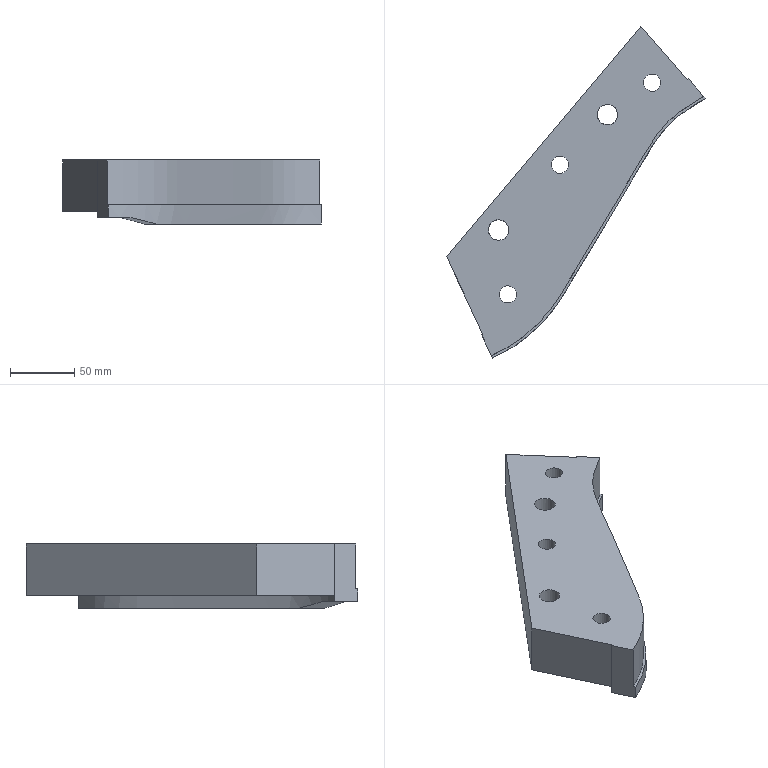Part | NX | features solid 2 | 1 solid | 25 faces | box 201.965 x 259.218 x 50 mm | volume 771440 mm3 | plane 14 | cylinder 8 | spline 3 | commonest cylinder face diameters 13.5 x3 19.5 x3 16 x2